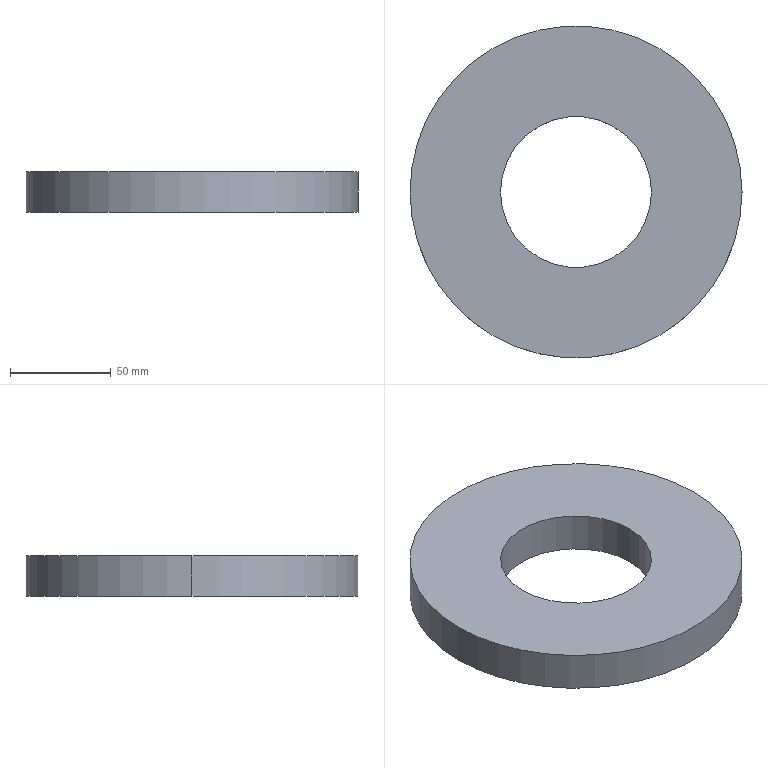Part | SolidWorks | features Extrusion 1 | 1 solid | 6 faces | box 165 x 165 x 20 mm | volume 339292 mm3 | cylinder 4 | plane 2 | commonest cylinder face diameters 75 x2 165 x2
STEP:
#1=CARTESIAN_POINT('',(-37.5,0.,20.));
#2=VERTEX_POINT('',#1);
#3=CARTESIAN_POINT('',(37.5,0.,20.));
#4=VERTEX_POINT('',#3);
#5=CARTESIAN_POINT('',(0.,0.,20.));
#6=DIRECTION('',(0.,0.,1.));
#7=DIRECTION('',(1.,0.,0.));
#8=AXIS2_PLACEMENT_3D('',#5,#6,#7);
#9=CIRCLE('',#8,37.5);
#10=EDGE_CURVE('',#2,#4,#9,.T.);
#11=ORIENTED_EDGE('',*,*,#10,.T.);
#12=CARTESIAN_POINT('',(37.5,0.,0.));
#13=VERTEX_POINT('',#12);
#14=CARTESIAN_POINT('',(37.5,0.,20.));
#15=DIRECTION('',(0.,0.,-1.));
#16=VECTOR('',#15,1000.);
#17=LINE('',#14,#16);
#18=EDGE_CURVE('',#4,#13,#17,.T.);
#19=ORIENTED_EDGE('',*,*,#18,.T.);
#20=CARTESIAN_POINT('',(-37.5,0.,0.));
#21=VERTEX_POINT('',#20);
#22=CARTESIAN_POINT('',(0.,0.,0.));
#23=DIRECTION('',(0.,0.,1.));
#24=DIRECTION('',(1.,0.,0.));
#25=AXIS2_PLACEMENT_3D('',#22,#23,#24);
#26=CIRCLE('',#25,37.5);
#27=EDGE_CURVE('',#21,#13,#26,.T.);
#28=ORIENTED_EDGE('',*,*,#27,.F.);
#29=CARTESIAN_POINT('',(-37.5,0.,20.));
#30=DIRECTION('',(0.,0.,-1.));
#31=VECTOR('',#30,1000.);
#32=LINE('',#29,#31);
#33=EDGE_CURVE('',#2,#21,#32,.T.);
#34=ORIENTED_EDGE('',*,*,#33,.F.);
#35=EDGE_LOOP('',(#11,#19,#28,#34));
#36=FACE_OUTER_BOUND('',#35,.T.);
#37=CARTESIAN_POINT('',(0.,0.,20.));
#38=DIRECTION('',(0.,0.,-1.));
#39=DIRECTION('',(-1.,0.,0.));
#40=AXIS2_PLACEMENT_3D('',#37,#38,#39);
#41=CYLINDRICAL_SURFACE('',#40,37.5);
#42=ADVANCED_FACE('',(#36),#41,.F.);
#43=CARTESIAN_POINT('',(82.5,0.,20.));
#44=VERTEX_POINT('',#43);
#45=CARTESIAN_POINT('',(-82.5,0.,20.));
#46=VERTEX_POINT('',#45);
#47=CARTESIAN_POINT('',(0.,0.,20.));
#48=DIRECTION('',(0.,0.,1.));
#49=DIRECTION('',(1.,0.,0.));
#50=AXIS2_PLACEMENT_3D('',#47,#48,#49);
#51=CIRCLE('',#50,82.5);
#52=EDGE_CURVE('',#44,#46,#51,.T.);
#53=ORIENTED_EDGE('',*,*,#52,.F.);
#54=CARTESIAN_POINT('',(82.5,0.,0.));
#55=VERTEX_POINT('',#54);
#56=CARTESIAN_POINT('',(82.5,0.,20.));
#57=DIRECTION('',(0.,0.,-1.));
#58=VECTOR('',#57,1000.);
#59=LINE('',#56,#58);
#60=EDGE_CURVE('',#44,#55,#59,.T.);
#61=ORIENTED_EDGE('',*,*,#60,.T.);
#62=CARTESIAN_POINT('',(-82.5,0.,0.));
#63=VERTEX_POINT('',#62);
#64=CARTESIAN_POINT('',(0.,0.,0.));
#65=DIRECTION('',(0.,0.,1.));
#66=DIRECTION('',(1.,0.,0.));
#67=AXIS2_PLACEMENT_3D('',#64,#65,#66);
#68=CIRCLE('',#67,82.5);
#69=EDGE_CURVE('',#55,#63,#68,.T.);
#70=ORIENTED_EDGE('',*,*,#69,.T.);
#71=CARTESIAN_POINT('',(-82.5,0.,20.));
#72=DIRECTION('',(0.,0.,-1.));
#73=VECTOR('',#72,1000.);
#74=LINE('',#71,#73);
#75=EDGE_CURVE('',#46,#63,#74,.T.);
#76=ORIENTED_EDGE('',*,*,#75,.F.);
#77=EDGE_LOOP('',(#53,#61,#70,#76));
#78=FACE_OUTER_BOUND('',#77,.T.);
#79=CARTESIAN_POINT('',(0.,0.,20.));
#80=DIRECTION('',(0.,0.,-1.));
#81=DIRECTION('',(-1.,0.,0.));
#82=AXIS2_PLACEMENT_3D('',#79,#80,#81);
#83=CYLINDRICAL_SURFACE('',#82,82.5);
#84=ADVANCED_FACE('',(#78),#83,.T.);
#85=CARTESIAN_POINT('',(0.,0.,20.));
#86=DIRECTION('',(0.,0.,1.));
#87=DIRECTION('',(1.,0.,0.));
#88=AXIS2_PLACEMENT_3D('',#85,#86,#87);
#89=CIRCLE('',#88,82.5);
#90=EDGE_CURVE('',#46,#44,#89,.T.);
#91=ORIENTED_EDGE('',*,*,#90,.T.);
#92=ORIENTED_EDGE('',*,*,#52,.T.);
#93=EDGE_LOOP('',(#91,#92));
#94=FACE_OUTER_BOUND('',#93,.T.);
#95=ORIENTED_EDGE('',*,*,#10,.F.);
#96=CARTESIAN_POINT('',(0.,0.,20.));
#97=DIRECTION('',(0.,0.,1.));
#98=DIRECTION('',(1.,0.,0.));
#99=AXIS2_PLACEMENT_3D('',#96,#97,#98);
#100=CIRCLE('',#99,37.5);
#101=EDGE_CURVE('',#4,#2,#100,.T.);
#102=ORIENTED_EDGE('',*,*,#101,.F.);
#103=EDGE_LOOP('',(#95,#102));
#104=FACE_BOUND('',#103,.T.);
#105=CARTESIAN_POINT('',(0.,0.,20.));
#106=DIRECTION('',(0.,0.,1.));
#107=DIRECTION('',(1.,0.,0.));
#108=AXIS2_PLACEMENT_3D('',#105,#106,#107);
#109=PLANE('',#108);
#110=ADVANCED_FACE('',(#94,#104),#109,.T.);
#111=CARTESIAN_POINT('',(0.,0.,0.));
#112=DIRECTION('',(0.,0.,1.));
#113=DIRECTION('',(1.,0.,0.));
#114=AXIS2_PLACEMENT_3D('',#111,#112,#113);
#115=CIRCLE('',#114,82.5);
#116=EDGE_CURVE('',#63,#55,#115,.T.);
#117=ORIENTED_EDGE('',*,*,#116,.F.);
#118=ORIENTED_EDGE('',*,*,#69,.F.);
#119=EDGE_LOOP('',(#117,#118));
#120=FACE_OUTER_BOUND('',#119,.T.);
#121=ORIENTED_EDGE('',*,*,#27,.T.);
#122=CARTESIAN_POINT('',(0.,0.,0.));
#123=DIRECTION('',(0.,0.,1.));
#124=DIRECTION('',(1.,0.,0.));
#125=AXIS2_PLACEMENT_3D('',#122,#123,#124);
#126=CIRCLE('',#125,37.5);
#127=EDGE_CURVE('',#13,#21,#126,.T.);
#128=ORIENTED_EDGE('',*,*,#127,.T.);
#129=EDGE_LOOP('',(#121,#128));
#130=FACE_BOUND('',#129,.T.);
#131=CARTESIAN_POINT('',(0.,0.,0.));
#132=DIRECTION('',(0.,0.,1.));
#133=DIRECTION('',(1.,0.,0.));
#134=AXIS2_PLACEMENT_3D('',#131,#132,#133);
#135=PLANE('',#134);
#136=ADVANCED_FACE('',(#120,#130),#135,.F.);
#137=ORIENTED_EDGE('',*,*,#60,.F.);
#138=ORIENTED_EDGE('',*,*,#90,.F.);
#139=ORIENTED_EDGE('',*,*,#75,.T.);
#140=ORIENTED_EDGE('',*,*,#116,.T.);
#141=EDGE_LOOP('',(#137,#138,#139,#140));
#142=FACE_OUTER_BOUND('',#141,.T.);
#143=CARTESIAN_POINT('',(0.,0.,20.));
#144=DIRECTION('',(0.,0.,-1.));
#145=DIRECTION('',(-1.,0.,0.));
#146=AXIS2_PLACEMENT_3D('',#143,#144,#145);
#147=CYLINDRICAL_SURFACE('',#146,82.5);
#148=ADVANCED_FACE('',(#142),#147,.T.);
#149=ORIENTED_EDGE('',*,*,#18,.F.);
#150=ORIENTED_EDGE('',*,*,#101,.T.);
#151=ORIENTED_EDGE('',*,*,#33,.T.);
#152=ORIENTED_EDGE('',*,*,#127,.F.);
#153=EDGE_LOOP('',(#149,#150,#151,#152));
#154=FACE_OUTER_BOUND('',#153,.T.);
#155=CARTESIAN_POINT('',(0.,0.,20.));
#156=DIRECTION('',(0.,0.,-1.));
#157=DIRECTION('',(-1.,0.,0.));
#158=AXIS2_PLACEMENT_3D('',#155,#156,#157);
#159=CYLINDRICAL_SURFACE('',#158,37.5);
#160=ADVANCED_FACE('',(#154),#159,.F.);
#161=CLOSED_SHELL('',(#42,#84,#110,#136,#148,#160));
#162=MANIFOLD_SOLID_BREP('',#161);
#163=CARTESIAN_POINT('',(0.,0.,0.));
#164=DIRECTION('',(0.,0.,1.));
#165=DIRECTION('',(1.,0.,0.));
#166=AXIS2_PLACEMENT_3D('',#163,#164,#165);
#167=(LENGTH_UNIT()NAMED_UNIT(*)SI_UNIT(.MILLI.,.METRE.));
#168=UNCERTAINTY_MEASURE_WITH_UNIT(LENGTH_MEASURE(0.00001),#167,'','');
#169=(NAMED_UNIT(*)PLANE_ANGLE_UNIT()SI_UNIT($,.RADIAN.));
#170=(NAMED_UNIT(*)SI_UNIT($,.STERADIAN.)SOLID_ANGLE_UNIT());
#171=(GEOMETRIC_REPRESENTATION_CONTEXT(3)GLOBAL_UNCERTAINTY_ASSIGNED_CONTEXT((#168))GLOBAL_UNIT_ASSIGNED_CONTEXT((#167,#169,#170))REPRESENTATION_CONTEXT('',''));
#172=ADVANCED_BREP_SHAPE_REPRESENTATION('',(#162,#166),#171);